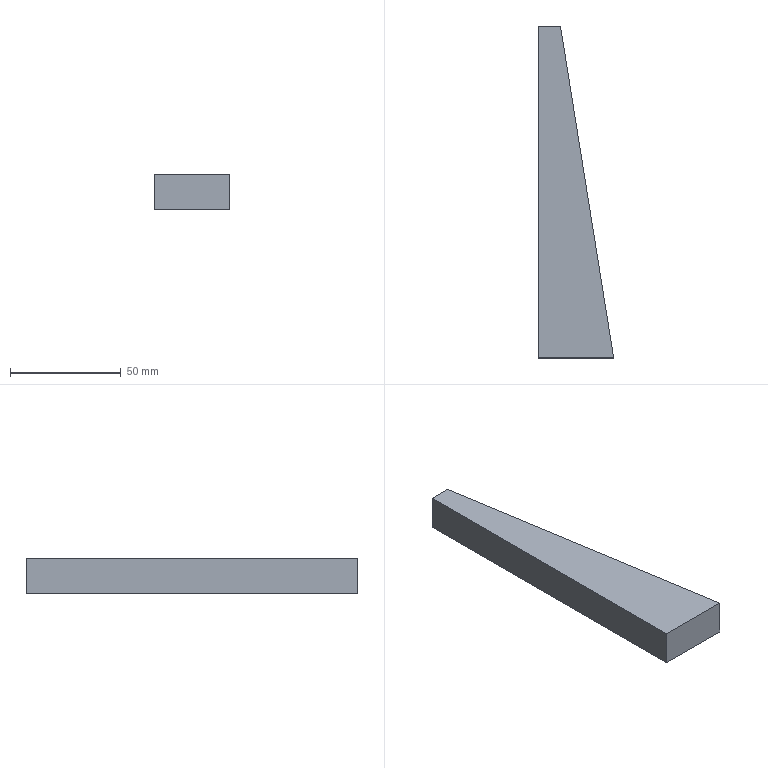Part | SolidWorks | features Extrusion 1 | 1 solid | 6 faces | box 34 x 150 x 16 mm | volume 52800 mm3 | plane 6
STEP:
#1=CARTESIAN_POINT('',(0.,150.,-8.));
#2=VERTEX_POINT('',#1);
#3=CARTESIAN_POINT('',(0.,0.,-8.));
#4=VERTEX_POINT('',#3);
#5=CARTESIAN_POINT('',(0.,0.,-8.));
#6=DIRECTION('',(0.,-1.,0.));
#7=VECTOR('',#6,1000.);
#8=LINE('',#5,#7);
#9=EDGE_CURVE('',#2,#4,#8,.T.);
#10=ORIENTED_EDGE('',*,*,#9,.T.);
#11=CARTESIAN_POINT('',(0.,0.,8.));
#12=VERTEX_POINT('',#11);
#13=CARTESIAN_POINT('',(0.,0.,8.));
#14=DIRECTION('',(0.,0.,-1.));
#15=VECTOR('',#14,1000.);
#16=LINE('',#13,#15);
#17=EDGE_CURVE('',#12,#4,#16,.T.);
#18=ORIENTED_EDGE('',*,*,#17,.F.);
#19=CARTESIAN_POINT('',(0.,150.,8.));
#20=VERTEX_POINT('',#19);
#21=CARTESIAN_POINT('',(0.,0.,8.));
#22=DIRECTION('',(0.,-1.,0.));
#23=VECTOR('',#22,1000.);
#24=LINE('',#21,#23);
#25=EDGE_CURVE('',#20,#12,#24,.T.);
#26=ORIENTED_EDGE('',*,*,#25,.F.);
#27=CARTESIAN_POINT('',(0.,150.,8.));
#28=DIRECTION('',(0.,0.,-1.));
#29=VECTOR('',#28,1000.);
#30=LINE('',#27,#29);
#31=EDGE_CURVE('',#20,#2,#30,.T.);
#32=ORIENTED_EDGE('',*,*,#31,.T.);
#33=EDGE_LOOP('',(#10,#18,#26,#32));
#34=FACE_OUTER_BOUND('',#33,.T.);
#35=CARTESIAN_POINT('',(0.,0.,8.));
#36=DIRECTION('',(1.,0.,0.));
#37=DIRECTION('',(0.,0.,-1.));
#38=AXIS2_PLACEMENT_3D('',#35,#36,#37);
#39=PLANE('',#38);
#40=ADVANCED_FACE('',(#34),#39,.F.);
#41=CARTESIAN_POINT('',(34.,0.,-8.));
#42=VERTEX_POINT('',#41);
#43=CARTESIAN_POINT('',(0.,0.,-8.));
#44=DIRECTION('',(1.,0.,0.));
#45=VECTOR('',#44,1000.);
#46=LINE('',#43,#45);
#47=EDGE_CURVE('',#4,#42,#46,.T.);
#48=ORIENTED_EDGE('',*,*,#47,.T.);
#49=CARTESIAN_POINT('',(34.,0.,8.));
#50=VERTEX_POINT('',#49);
#51=CARTESIAN_POINT('',(34.,0.,8.));
#52=DIRECTION('',(0.,0.,-1.));
#53=VECTOR('',#52,1000.);
#54=LINE('',#51,#53);
#55=EDGE_CURVE('',#50,#42,#54,.T.);
#56=ORIENTED_EDGE('',*,*,#55,.F.);
#57=CARTESIAN_POINT('',(0.,0.,8.));
#58=DIRECTION('',(1.,0.,0.));
#59=VECTOR('',#58,1000.);
#60=LINE('',#57,#59);
#61=EDGE_CURVE('',#12,#50,#60,.T.);
#62=ORIENTED_EDGE('',*,*,#61,.F.);
#63=ORIENTED_EDGE('',*,*,#17,.T.);
#64=EDGE_LOOP('',(#48,#56,#62,#63));
#65=FACE_OUTER_BOUND('',#64,.T.);
#66=CARTESIAN_POINT('',(0.,0.,8.));
#67=DIRECTION('',(0.,1.,0.));
#68=DIRECTION('',(0.,0.,1.));
#69=AXIS2_PLACEMENT_3D('',#66,#67,#68);
#70=PLANE('',#69);
#71=ADVANCED_FACE('',(#65),#70,.F.);
#72=CARTESIAN_POINT('',(10.,150.,-8.));
#73=VERTEX_POINT('',#72);
#74=CARTESIAN_POINT('',(10.,150.,-8.));
#75=DIRECTION('',(-0.158,0.9874,0.));
#76=VECTOR('',#75,1000.);
#77=LINE('',#74,#76);
#78=EDGE_CURVE('',#42,#73,#77,.T.);
#79=ORIENTED_EDGE('',*,*,#78,.T.);
#80=CARTESIAN_POINT('',(10.,150.,8.));
#81=VERTEX_POINT('',#80);
#82=CARTESIAN_POINT('',(10.,150.,8.));
#83=DIRECTION('',(0.,0.,-1.));
#84=VECTOR('',#83,1000.);
#85=LINE('',#82,#84);
#86=EDGE_CURVE('',#81,#73,#85,.T.);
#87=ORIENTED_EDGE('',*,*,#86,.F.);
#88=CARTESIAN_POINT('',(10.,150.,8.));
#89=DIRECTION('',(-0.158,0.9874,0.));
#90=VECTOR('',#89,1000.);
#91=LINE('',#88,#90);
#92=EDGE_CURVE('',#50,#81,#91,.T.);
#93=ORIENTED_EDGE('',*,*,#92,.F.);
#94=ORIENTED_EDGE('',*,*,#55,.T.);
#95=EDGE_LOOP('',(#79,#87,#93,#94));
#96=FACE_OUTER_BOUND('',#95,.T.);
#97=CARTESIAN_POINT('',(10.,150.,8.));
#98=DIRECTION('',(-0.9874,-0.158,0.));
#99=DIRECTION('',(0.158,-0.9874,0.));
#100=AXIS2_PLACEMENT_3D('',#97,#98,#99);
#101=PLANE('',#100);
#102=ADVANCED_FACE('',(#96),#101,.F.);
#103=CARTESIAN_POINT('',(0.,150.,-8.));
#104=DIRECTION('',(-1.,0.,0.));
#105=VECTOR('',#104,1000.);
#106=LINE('',#103,#105);
#107=EDGE_CURVE('',#73,#2,#106,.T.);
#108=ORIENTED_EDGE('',*,*,#107,.T.);
#109=ORIENTED_EDGE('',*,*,#31,.F.);
#110=CARTESIAN_POINT('',(0.,150.,8.));
#111=DIRECTION('',(-1.,0.,0.));
#112=VECTOR('',#111,1000.);
#113=LINE('',#110,#112);
#114=EDGE_CURVE('',#81,#20,#113,.T.);
#115=ORIENTED_EDGE('',*,*,#114,.F.);
#116=ORIENTED_EDGE('',*,*,#86,.T.);
#117=EDGE_LOOP('',(#108,#109,#115,#116));
#118=FACE_OUTER_BOUND('',#117,.T.);
#119=CARTESIAN_POINT('',(0.,150.,8.));
#120=DIRECTION('',(0.,-1.,0.));
#121=DIRECTION('',(0.,0.,-1.));
#122=AXIS2_PLACEMENT_3D('',#119,#120,#121);
#123=PLANE('',#122);
#124=ADVANCED_FACE('',(#118),#123,.F.);
#125=ORIENTED_EDGE('',*,*,#25,.T.);
#126=ORIENTED_EDGE('',*,*,#61,.T.);
#127=ORIENTED_EDGE('',*,*,#92,.T.);
#128=ORIENTED_EDGE('',*,*,#114,.T.);
#129=EDGE_LOOP('',(#125,#126,#127,#128));
#130=FACE_OUTER_BOUND('',#129,.T.);
#131=CARTESIAN_POINT('',(0.,150.,8.));
#132=DIRECTION('',(0.,0.,-1.));
#133=DIRECTION('',(-1.,0.,0.));
#134=AXIS2_PLACEMENT_3D('',#131,#132,#133);
#135=PLANE('',#134);
#136=ADVANCED_FACE('',(#130),#135,.F.);
#137=ORIENTED_EDGE('',*,*,#9,.F.);
#138=ORIENTED_EDGE('',*,*,#107,.F.);
#139=ORIENTED_EDGE('',*,*,#78,.F.);
#140=ORIENTED_EDGE('',*,*,#47,.F.);
#141=EDGE_LOOP('',(#137,#138,#139,#140));
#142=FACE_OUTER_BOUND('',#141,.T.);
#143=CARTESIAN_POINT('',(0.,150.,-8.));
#144=DIRECTION('',(0.,0.,-1.));
#145=DIRECTION('',(-1.,0.,0.));
#146=AXIS2_PLACEMENT_3D('',#143,#144,#145);
#147=PLANE('',#146);
#148=ADVANCED_FACE('',(#142),#147,.T.);
#149=CLOSED_SHELL('',(#40,#71,#102,#124,#136,#148));
#150=MANIFOLD_SOLID_BREP('',#149);
#151=CARTESIAN_POINT('',(0.,0.,0.));
#152=DIRECTION('',(0.,0.,1.));
#153=DIRECTION('',(1.,0.,0.));
#154=AXIS2_PLACEMENT_3D('',#151,#152,#153);
#155=(LENGTH_UNIT()NAMED_UNIT(*)SI_UNIT(.MILLI.,.METRE.));
#156=UNCERTAINTY_MEASURE_WITH_UNIT(LENGTH_MEASURE(0.00001),#155,'','');
#157=(NAMED_UNIT(*)PLANE_ANGLE_UNIT()SI_UNIT($,.RADIAN.));
#158=(NAMED_UNIT(*)SI_UNIT($,.STERADIAN.)SOLID_ANGLE_UNIT());
#159=(GEOMETRIC_REPRESENTATION_CONTEXT(3)GLOBAL_UNCERTAINTY_ASSIGNED_CONTEXT((#156))GLOBAL_UNIT_ASSIGNED_CONTEXT((#155,#157,#158))REPRESENTATION_CONTEXT('',''));
#160=ADVANCED_BREP_SHAPE_REPRESENTATION('',(#150,#154),#159);